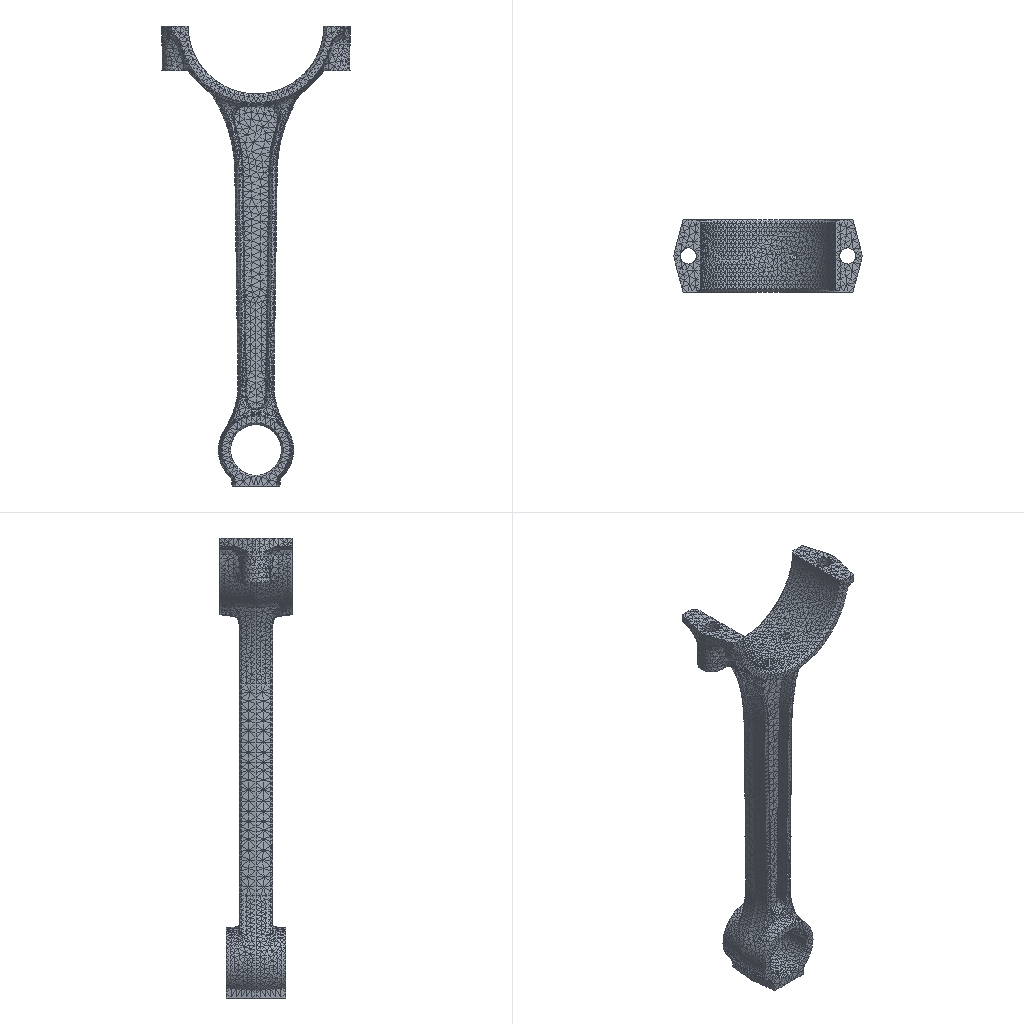Simulation study | ansys workbench
Set-up summary:
category,name,step,type,value,unit,region
solver,ansys_workbench
units,SI m-kg-s (Pa),,stated,"/units,MKS"
analysis,LS1,,static
load_step,LS1,LS1,static,nsubst=1; time=1
mesh,nodes,,,49445
mesh,elements,,,29544
element_type,SOLID187,,,28251
element_type,SURF154,,,1293
material,Structural Steel,,E,2e+11,Pa
material,Structural Steel,,nu,0.3
material,Structural Steel,,density,7850,kg m^-3
material,Structural Steel,,conductivity,60.5,W m^-1 C^-1
material,Structural Steel,,specific_heat,434,J kg^-1 C^-1
material,Structural Steel,,cte,1.2e-05,C^-1
material,Structural Steel,,permeability,10000
material,Structural Steel,,resistivity,1.7e-07,kg m^3 A^-2 s^-3
load,Define Force Using Surface Effect Elements,LS1,surface-effect pres face 3,-1.45199e+06,,SURF154 #2
bc,Fixed Supports,model,fixed,[dofs=ALL],,_FIXEDSU
bc,Frictionless Supports X,model,fixed,[dofs=UX],,_FRICSUX
named_set,_FIXEDSU,,node,885
named_set,_FRICSUX,,node,454
Ansys APDL input file, long lists of numbers shortened:
/batch
/config,noeldb,1     ! force off writing results to database
*get,_wallstrt,active,,time,wall
! ANSYS input file written by Workbench version 2025 R2
! File used for geometry attach:
/title,wbnew--____ (A5)
! ****** Begin Custom Load Command Snippet ******
/COM, ACT Extensions:
/COM,     LSDYNA, 2025.2
/COM,/COM,     ANSYSMotion, 2025.2
/COM,
! ****** End   Custom Load Command Snippet ******
*DIM,_wb_ProjectScratch_dir,string,248
_wb_ProjectScratch_dir(1) = ''
*DIM,_wb_SolverFiles_dir,string,248
_wb_SolverFiles_dir(1) = ''
*DIM,_wb_userfiles_dir,string,248
_wb_userfiles_dir(1) = ''
/com,--- Data in consistent MKS units. See Solving Units in the help system for more information.
/units,MKS
/nopr
/wb,file,start              !  signify a WB generated input file
/prep7
! Turn off shape checking because checks already performed inside WB mesher.
! See help system for more information.
SHPP,OFF,,NOWARN
/nolist
etcon,set             ! allow ANSYS to choose best KEYOP's for 180x elements, resets any applicable keyopt to MAPDL defaults
/com,*********** Send User Defined Coordinate System(s) ***********
csys,0
/com,*********** Nodes for the whole assembly ***********
nblock,3,,54389
(1i9,3e20.9e3)
        1     1.972527442E-02     1.120369928E-18     1.656077353E-01
! (49444 more lines like these left out)
-1
/wb,elem,start            !  set before creation of elements
/com,*********** Elements for Body 1 'Part 1' ***********
et,1,187
MAT,1 $ TYPE,1 $ REAL,1 $ SECNUM,1 $ ESYS,0
eblock,11,COMPACT,,28251
(11i9)
        1     4064     4118     7756     6288    33519    33880    33522    33520    33876    45954
! (28250 more lines like these left out)
-1
secnum,1    ! reset the section ID to default
/wb,elem,end               !  done creating elements
toffst,273.15,      ! Temperature offset from absolute zero
/com,*********** Set Reference Temperature ***********
tref,22.
/wb,mat,start              !  starting to send materials
/com,*********** Send Materials ***********
Temperature = 'TEMP' ! Temperature
MP,DENS,1,7850,	! kg m^-3
MP,ALPX,1,1.2e-05,	! C^-1
MP,C,1,434,	! J kg^-1 C^-1
MP,KXX,1,60.5,	! W m^-1 C^-1
MP,RSVX,1,1.7e-07,	! kg m^3 A^-2 s^-3
MP,EX,1,200000000000,	! Pa
MP,NUXY,1,0.3,
MP,MURX,1,10000,
/wb,mat,end                !  done sending materials
!************************* Model Summary ********************
!Part 1,	结构钢,	matid,	1
!************************* End Model Summary ********************
! get the diagonal of the bounding box. Needed later for other things
*get,_xmin,node,,mnloc,x
*get,_ymin,node,,mnloc,y
*get,_zmin,node,,mnloc,z
*get,_xmax,node,,mxloc,x
*get,_ymax,node,,mxloc,y
*get,_zmax,node,,mxloc,z
_ASMDIAG=(_xmax-_xmin)*(_xmax-_xmin)+(_ymax-_ymin)*(_ymax-_ymin)+(_zmax-_zmin)*(_zmax-_zmin)
_ASMDIAG=SQRT(_ASMDIAG)
/wb,contact,start          !  starting to send contact
/wb,contact,end            !  done creating contacts
/golist
/wb,load,start             !  starting to send loads
/com,*********** Fixed Supports ***********
CMBLOCK,_FIXEDSU,NODE,      885
(8i10)
      2318     -2387      3820     -4206     24158     24159     24162    -24164
! (110 more lines like these left out)
cmsel,s,_FIXEDSU
d,all,all
nsel,all
/com,********* Frictionless Supports X *********
CMBLOCK,_FRICSUX,NODE,      454
(8i10)
       461      -471       493      -503       754      -764      2247     -2257
! (56 more lines like these left out)
cmsel,s,_FRICSUX
d,all,ux,0
nsel,all
/com,*********** Node Rotations ***********
nmod,462,,,,-32.727,0.,0.
nmod,463,,,,-65.455,0.,0.
nmod,464,,,,-98.182,0.,0.
nmod,465,,,,-130.909,0.,0.
! (868 more lines like these left out)
/com,*********** Define Force Using Surface Effect Elements ***********
local,12,0,0.,0.,0.,0.,0.,0.
csys,0
et,2,154
MAT,2 $ TYPE,2 $ REAL,2 $ SECNUM,2 $ ESYS,12
eblock,11,COMPACT,,1293
(11i9)
    39596       83       84     4220     4220     8390     8399     4220     8394
! (1292 more lines like these left out)
-1
secnum,1    ! reset the section ID to default
esel,s,type,,2
keyop,2,2,1         ! Apply load in local coordinate system
keyop,2,7,1         ! Use original area so load is constant in large deformation
esel,all
/gst,on,on
fini
*get,_numnode,node,0,count
*get,_numelem,elem,0,count
*get, _MAXELEMNUM, elem, 0, NUM, MAX
*get, _MAXNODENUM, node, 0, NUM, MAX
*get, _MAXELEMTYPE, etyp, 0, NUM, MAX
*get, _MAXREALCONST, rcon, 0, NUM, MAX
/go
/wb,load,end               !  done creating loads
/com,--- Number of total nodes = %_numnode%
/com,--- Number of contact elements = 1293
/com,--- Number of spring elements = 0
/com,--- Number of bearing elements = 0
/com,--- Number of solid elements = 28251
/com,--- Number of condensed parts = 0
/com,--- Number of total elements = %_numelem%
*get,_wallbsol,active,,time,wall
/com,****************************************************************************
/com,*************************    SOLUTION       ********************************
/com,****************************************************************************
/solu
antype,0                   ! static analysis
_thickRatio=  1     ! Ratio of thick parts in the model
eqsl,pcg,1e-8,,,,,,1
cntr,print,1               ! print out contact info and also make no initial contact an error
cncheck,dmp		!	Enable program controlled contact splitting for distributed memory parallel run
dmpoption,emat,no             ! Don't combine emat file for DANSYS
dmpoption,esav,no             ! Don't combine esav file for DANSYS
nldiag,cont,iter           ! print out contact info each equilibrium iteration
rescontrol,,none                 ! Do not keep any restart files
/com,****************************************************
/com,******************* SOLVE FOR LS 1 OF 1 ****************
esel,s,type,,2
nsle
sfe,all,1,pres,1,0.
sfe,all,2,pres,1,0.
sfe,all,3,pres,1,-1451992.61
nsel,all
esel,all
/nopr
/gopr
nsub,1,1,1
time,1.
outres,erase
outres,all,none
outres,nsol,all,
outres,rsol,all
outres,eangl,all
outres,etmp,all
outres,veng,all
outres,strs,all,
outres,epel,all,
outres,eppl,all,
outres,cont,all,
! *********** WB SOLVE COMMAND ***********
! check interactive state
*get,ANSINTER_,active,,int
*if,ANSINTER_,ne,0,then
/eof
*endif
solve
/com *************** Write FE CONNECTORS *********
CEWRITE,file,ce,,INTE
/com,****************************************************
/com,*************** FINISHED SOLVE FOR LS 1 *************
*get,_wallasol,active,,time,wall
/nopr
*get,_numnode,node,0,count
*get,_numelem,elem,0,count
*get, _MAXELEMNUM, elem, 0, NUM, MAX
*get, _MAXNODENUM, node, 0, NUM, MAX,,,INTERNAL
*get, _MAXELEMTYPE, etyp, 0, NUM, MAX
*get, _MAXREALCONST, rcon, 0, NUM, MAX
*get,_NSOLTHREADS,active,0,ntfs
*get,_NSOLPROCESSES,active,0,npfs
/gopr
*get,_PCGITER,active,,solu,cgiter
/post1
xmlo,ENCODING,ISO-8859-1
xmlo,parm
/xml,parm,xml
fini
/gopr
*get,_walldone,active,,time,wall
_preptime=(_wallbsol-_wallstrt)*3600
_solvtime=(_wallasol-_wallbsol)*3600
_posttime=(_walldone-_wallasol)*3600
_totaltim=(_walldone-_wallstrt)*3600
*get,_dlbratio,active,0,solu,dlbr
*get,_combtime,active,0,solu,comb
*get,_ssmode,active,0,solu,ssmm
*get,_ndofs,active,0,solu,ndof
*get,_sol_end_time,active,0,set,time
*if,_sol_end_time,eq,1.,then
/fclean				!clean distributed files
*endif
/com,--- Total number of nodes = %_numnode%
/com,--- Total number of elements = %_numelem%
/com,--- Element load balance ratio = %_dlbratio%
/com,--- Time to combine distributed files = %_combtime%
/com,--- Sparse memory mode = %_ssmode%
/com,--- Number of DOF = %_ndofs%
/wb,file,end               ! done with WB generated input
Results summary:
result,analyses[0].index,,,1
result,analyses[0].system,,,SYS
result,analyses[0].deck,,,deck.dat
result,analyses[0].solve_status,,,completed
result,analyses[0].analysis_type,,,static
result,analyses[0].physics,,,mechanical
result,analyses[0].unit_system,,,"MKS: m, kg, N, s, V, A, degC"
result,analyses[0].n_sets,,,1
result,analyses[0].load_steps[0].set,set=1,,1
result,analyses[0].load_steps[0].time_or_freq,set=1,,1
result,analyses[0].load_steps[0].max_displacement_magnitude,set=1,,2.76029e-05
result,analyses[0].load_steps[0].max_von_mises_nodal,set=1,,5.43234e+07
result,analyses[0].load_steps[0].reaction_force_sum_xyz[1],set=1,,1.00751e-06
result,analyses[0].load_steps[0].reaction_force_sum_xyz[2],set=1,,-6.28364e-07
result,analyses[0].load_steps[0].reaction_force_sum_xyz[3],set=1,,4500